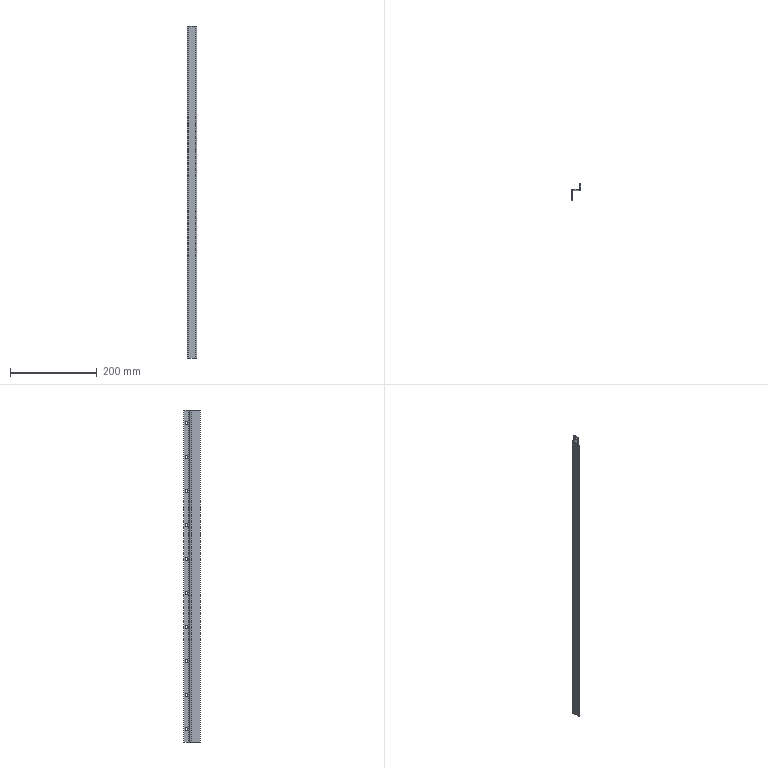Part | NX | features solid 2 | 1 solid | 34 faces | box 22 x 38 x 765 mm | volume 84234 mm3 | cylinder 24 | plane 10 | commonest cylinder face diameters 6 x20 4 x2 8 x2
STEP:
#1=CARTESIAN_POINT('',(2193.,-769.,290.));
#2=VERTEX_POINT('',#1);
#3=CARTESIAN_POINT('',(2191.,-769.,290.));
#4=VERTEX_POINT('',#3);
#5=CARTESIAN_POINT('',(2957.259,-769.,290.));
#6=DIRECTION('',(-1.,0.,0.));
#7=VECTOR('',#6,1000.);
#8=LINE('',#5,#7);
#9=EDGE_CURVE('',#2,#4,#8,.T.);
#10=ORIENTED_EDGE('',*,*,#9,.F.);
#11=CARTESIAN_POINT('',(2193.,-763.,290.));
#12=VERTEX_POINT('',#11);
#13=CARTESIAN_POINT('',(2193.,-766.,290.));
#14=DIRECTION('',(-1.,0.,0.));
#15=DIRECTION('',(0.,1.,0.));
#16=AXIS2_PLACEMENT_3D('',#13,#14,#15);
#17=CIRCLE('',#16,3.);
#18=EDGE_CURVE('',#12,#2,#17,.T.);
#19=ORIENTED_EDGE('',*,*,#18,.F.);
#20=CARTESIAN_POINT('',(2191.,-763.,290.));
#21=VERTEX_POINT('',#20);
#22=CARTESIAN_POINT('',(2957.259,-763.,290.));
#23=DIRECTION('',(-1.,0.,0.));
#24=VECTOR('',#23,1000.);
#25=LINE('',#22,#24);
#26=EDGE_CURVE('',#21,#12,#25,.F.);
#27=ORIENTED_EDGE('',*,*,#26,.F.);
#28=CARTESIAN_POINT('',(2191.,-766.,290.));
#29=DIRECTION('',(-1.,0.,0.));
#30=DIRECTION('',(0.,0.,1.));
#31=AXIS2_PLACEMENT_3D('',#28,#29,#30);
#32=CIRCLE('',#31,3.);
#33=EDGE_CURVE('',#21,#4,#32,.T.);
#34=ORIENTED_EDGE('',*,*,#33,.T.);
#35=EDGE_LOOP('',(#10,#19,#27,#34));
#36=FACE_BOUND('',#35,.T.);
#37=CARTESIAN_POINT('',(2957.259,-766.,290.));
#38=DIRECTION('',(-1.,0.,0.));
#39=DIRECTION('',(0.,1.,0.));
#40=AXIS2_PLACEMENT_3D('',#37,#38,#39);
#41=CYLINDRICAL_SURFACE('',#40,3.);
#42=ADVANCED_FACE('',(#36),#41,.F.);
#43=CARTESIAN_POINT('',(2173.,-777.,1025.));
#44=VERTEX_POINT('',#43);
#45=CARTESIAN_POINT('',(2173.,-798.,1025.));
#46=VERTEX_POINT('',#45);
#47=CARTESIAN_POINT('',(2173.,-775.,1025.));
#48=DIRECTION('',(0.,-1.,0.));
#49=VECTOR('',#48,1000.);
#50=LINE('',#47,#49);
#51=EDGE_CURVE('',#44,#46,#50,.T.);
#52=ORIENTED_EDGE('',*,*,#51,.T.);
#53=CARTESIAN_POINT('',(2173.,-798.,260.));
#54=VERTEX_POINT('',#53);
#55=CARTESIAN_POINT('',(2173.,-798.,260.));
#56=DIRECTION('',(0.,0.,1.));
#57=VECTOR('',#56,1000.);
#58=LINE('',#55,#57);
#59=EDGE_CURVE('',#54,#46,#58,.T.);
#60=ORIENTED_EDGE('',*,*,#59,.F.);
#61=CARTESIAN_POINT('',(2173.,-777.,260.));
#62=VERTEX_POINT('',#61);
#63=CARTESIAN_POINT('',(2173.,-775.,260.));
#64=DIRECTION('',(0.,-1.,0.));
#65=VECTOR('',#64,1000.);
#66=LINE('',#63,#65);
#67=EDGE_CURVE('',#62,#54,#66,.T.);
#68=ORIENTED_EDGE('',*,*,#67,.F.);
#69=CARTESIAN_POINT('',(2173.,-777.,260.));
#70=DIRECTION('',(0.,0.,1.));
#71=VECTOR('',#70,1000.);
#72=LINE('',#69,#71);
#73=EDGE_CURVE('',#62,#44,#72,.T.);
#74=ORIENTED_EDGE('',*,*,#73,.T.);
#75=EDGE_LOOP('',(#52,#60,#68,#74));
#76=FACE_BOUND('',#75,.T.);
#77=CARTESIAN_POINT('',(2173.,-775.,260.));
#78=DIRECTION('',(-1.,0.,0.));
#79=DIRECTION('',(0.,0.,1.));
#80=AXIS2_PLACEMENT_3D('',#77,#78,#79);
#81=PLANE('',#80);
#82=ADVANCED_FACE('',(#76),#81,.F.);
#83=CARTESIAN_POINT('',(2175.,-775.,1025.));
#84=VERTEX_POINT('',#83);
#85=CARTESIAN_POINT('',(2175.,-777.,1025.));
#86=DIRECTION('',(0.,0.,1.));
#87=DIRECTION('',(0.,1.,0.));
#88=AXIS2_PLACEMENT_3D('',#85,#86,#87);
#89=CIRCLE('',#88,2.);
#90=EDGE_CURVE('',#84,#44,#89,.T.);
#91=ORIENTED_EDGE('',*,*,#90,.T.);
#92=ORIENTED_EDGE('',*,*,#73,.F.);
#93=CARTESIAN_POINT('',(2175.,-775.,260.));
#94=VERTEX_POINT('',#93);
#95=CARTESIAN_POINT('',(2175.,-777.,260.));
#96=DIRECTION('',(0.,0.,1.));
#97=DIRECTION('',(0.,1.,0.));
#98=AXIS2_PLACEMENT_3D('',#95,#96,#97);
#99=CIRCLE('',#98,2.);
#100=EDGE_CURVE('',#94,#62,#99,.T.);
#101=ORIENTED_EDGE('',*,*,#100,.F.);
#102=CARTESIAN_POINT('',(2175.,-775.,260.));
#103=DIRECTION('',(0.,0.,1.));
#104=VECTOR('',#103,1000.);
#105=LINE('',#102,#104);
#106=EDGE_CURVE('',#94,#84,#105,.T.);
#107=ORIENTED_EDGE('',*,*,#106,.T.);
#108=EDGE_LOOP('',(#91,#92,#101,#107));
#109=FACE_BOUND('',#108,.T.);
#110=CARTESIAN_POINT('',(2175.,-777.,260.));
#111=DIRECTION('',(0.,0.,1.));
#112=DIRECTION('',(0.,-1.,0.));
#113=AXIS2_PLACEMENT_3D('',#110,#111,#112);
#114=CYLINDRICAL_SURFACE('',#113,2.);
#115=ADVANCED_FACE('',(#109),#114,.F.);
#116=CARTESIAN_POINT('',(2189.,-775.,1025.));
#117=VERTEX_POINT('',#116);
#118=CARTESIAN_POINT('',(2193.,-775.,1025.));
#119=DIRECTION('',(-1.,0.,0.));
#120=VECTOR('',#119,1000.);
#121=LINE('',#118,#120);
#122=EDGE_CURVE('',#117,#84,#121,.T.);
#123=ORIENTED_EDGE('',*,*,#122,.T.);
#124=ORIENTED_EDGE('',*,*,#106,.F.);
#125=CARTESIAN_POINT('',(2189.,-775.,260.));
#126=VERTEX_POINT('',#125);
#127=CARTESIAN_POINT('',(2193.,-775.,260.));
#128=DIRECTION('',(-1.,0.,0.));
#129=VECTOR('',#128,1000.);
#130=LINE('',#127,#129);
#131=EDGE_CURVE('',#126,#94,#130,.T.);
#132=ORIENTED_EDGE('',*,*,#131,.F.);
#133=CARTESIAN_POINT('',(2189.,-775.,260.));
#134=DIRECTION('',(0.,0.,1.));
#135=VECTOR('',#134,1000.);
#136=LINE('',#133,#135);
#137=EDGE_CURVE('',#126,#117,#136,.T.);
#138=ORIENTED_EDGE('',*,*,#137,.T.);
#139=EDGE_LOOP('',(#123,#124,#132,#138));
#140=FACE_BOUND('',#139,.T.);
#141=CARTESIAN_POINT('',(2193.,-775.,260.));
#142=DIRECTION('',(0.,1.,0.));
#143=DIRECTION('',(0.,0.,-1.));
#144=AXIS2_PLACEMENT_3D('',#141,#142,#143);
#145=PLANE('',#144);
#146=ADVANCED_FACE('',(#140),#145,.F.);
#147=CARTESIAN_POINT('',(2193.,-771.,1025.));
#148=VERTEX_POINT('',#147);
#149=CARTESIAN_POINT('',(2189.,-771.,1025.));
#150=DIRECTION('',(0.,0.,-1.));
#151=DIRECTION('',(0.,-1.,0.));
#152=AXIS2_PLACEMENT_3D('',#149,#150,#151);
#153=CIRCLE('',#152,4.);
#154=EDGE_CURVE('',#148,#117,#153,.T.);
#155=ORIENTED_EDGE('',*,*,#154,.T.);
#156=ORIENTED_EDGE('',*,*,#137,.F.);
#157=CARTESIAN_POINT('',(2193.,-771.,260.));
#158=VERTEX_POINT('',#157);
#159=CARTESIAN_POINT('',(2189.,-771.,260.));
#160=DIRECTION('',(0.,0.,-1.));
#161=DIRECTION('',(0.,-1.,0.));
#162=AXIS2_PLACEMENT_3D('',#159,#160,#161);
#163=CIRCLE('',#162,4.);
#164=EDGE_CURVE('',#158,#126,#163,.T.);
#165=ORIENTED_EDGE('',*,*,#164,.F.);
#166=CARTESIAN_POINT('',(2193.,-771.,260.));
#167=DIRECTION('',(0.,0.,1.));
#168=VECTOR('',#167,1000.);
#169=LINE('',#166,#168);
#170=EDGE_CURVE('',#158,#148,#169,.T.);
#171=ORIENTED_EDGE('',*,*,#170,.T.);
#172=EDGE_LOOP('',(#155,#156,#165,#171));
#173=FACE_BOUND('',#172,.T.);
#174=CARTESIAN_POINT('',(2189.,-771.,260.));
#175=DIRECTION('',(0.,0.,1.));
#176=DIRECTION('',(0.,-1.,0.));
#177=AXIS2_PLACEMENT_3D('',#174,#175,#176);
#178=CYLINDRICAL_SURFACE('',#177,4.);
#179=ADVANCED_FACE('',(#173),#178,.T.);
#180=ORIENTED_EDGE('',*,*,#18,.T.);
#181=CARTESIAN_POINT('',(2193.,-766.,290.));
#182=DIRECTION('',(-1.,0.,0.));
#183=DIRECTION('',(0.,1.,0.));
#184=AXIS2_PLACEMENT_3D('',#181,#182,#183);
#185=CIRCLE('',#184,3.);
#186=EDGE_CURVE('',#2,#12,#185,.T.);
#187=ORIENTED_EDGE('',*,*,#186,.T.);
#188=EDGE_LOOP('',(#180,#187));
#189=FACE_BOUND('',#188,.T.);
#190=CARTESIAN_POINT('',(2193.,-763.,368.333));
#191=VERTEX_POINT('',#190);
#192=CARTESIAN_POINT('',(2193.,-769.,368.333));
#193=VERTEX_POINT('',#192);
#194=CARTESIAN_POINT('',(2193.,-766.,368.333));
#195=DIRECTION('',(-1.,0.,0.));
#196=DIRECTION('',(0.,1.,0.));
#197=AXIS2_PLACEMENT_3D('',#194,#195,#196);
#198=CIRCLE('',#197,3.);
#199=EDGE_CURVE('',#191,#193,#198,.T.);
#200=ORIENTED_EDGE('',*,*,#199,.T.);
#201=CARTESIAN_POINT('',(2193.,-766.,368.333));
#202=DIRECTION('',(-1.,0.,0.));
#203=DIRECTION('',(0.,1.,0.));
#204=AXIS2_PLACEMENT_3D('',#201,#202,#203);
#205=CIRCLE('',#204,3.);
#206=EDGE_CURVE('',#193,#191,#205,.T.);
#207=ORIENTED_EDGE('',*,*,#206,.T.);
#208=EDGE_LOOP('',(#200,#207));
#209=FACE_BOUND('',#208,.T.);
#210=CARTESIAN_POINT('',(2193.,-763.,446.667));
#211=VERTEX_POINT('',#210);
#212=CARTESIAN_POINT('',(2193.,-769.,446.667));
#213=VERTEX_POINT('',#212);
#214=CARTESIAN_POINT('',(2193.,-766.,446.667));
#215=DIRECTION('',(-1.,0.,0.));
#216=DIRECTION('',(0.,1.,0.));
#217=AXIS2_PLACEMENT_3D('',#214,#215,#216);
#218=CIRCLE('',#217,3.);
#219=EDGE_CURVE('',#211,#213,#218,.T.);
#220=ORIENTED_EDGE('',*,*,#219,.T.);
#221=CARTESIAN_POINT('',(2193.,-766.,446.667));
#222=DIRECTION('',(-1.,0.,0.));
#223=DIRECTION('',(0.,1.,0.));
#224=AXIS2_PLACEMENT_3D('',#221,#222,#223);
#225=CIRCLE('',#224,3.);
#226=EDGE_CURVE('',#213,#211,#225,.T.);
#227=ORIENTED_EDGE('',*,*,#226,.T.);
#228=EDGE_LOOP('',(#220,#227));
#229=FACE_BOUND('',#228,.T.);
#230=CARTESIAN_POINT('',(2193.,-763.,525.));
#231=VERTEX_POINT('',#230);
#232=CARTESIAN_POINT('',(2193.,-769.,525.));
#233=VERTEX_POINT('',#232);
#234=CARTESIAN_POINT('',(2193.,-766.,525.));
#235=DIRECTION('',(-1.,0.,0.));
#236=DIRECTION('',(0.,1.,0.));
#237=AXIS2_PLACEMENT_3D('',#234,#235,#236);
#238=CIRCLE('',#237,3.);
#239=EDGE_CURVE('',#231,#233,#238,.T.);
#240=ORIENTED_EDGE('',*,*,#239,.T.);
#241=CARTESIAN_POINT('',(2193.,-766.,525.));
#242=DIRECTION('',(-1.,0.,0.));
#243=DIRECTION('',(0.,1.,0.));
#244=AXIS2_PLACEMENT_3D('',#241,#242,#243);
#245=CIRCLE('',#244,3.);
#246=EDGE_CURVE('',#233,#231,#245,.T.);
#247=ORIENTED_EDGE('',*,*,#246,.T.);
#248=EDGE_LOOP('',(#240,#247));
#249=FACE_BOUND('',#248,.T.);
#250=CARTESIAN_POINT('',(2193.,-763.,603.333));
#251=VERTEX_POINT('',#250);
#252=CARTESIAN_POINT('',(2193.,-769.,603.333));
#253=VERTEX_POINT('',#252);
#254=CARTESIAN_POINT('',(2193.,-766.,603.333));
#255=DIRECTION('',(-1.,0.,0.));
#256=DIRECTION('',(0.,1.,0.));
#257=AXIS2_PLACEMENT_3D('',#254,#255,#256);
#258=CIRCLE('',#257,3.);
#259=EDGE_CURVE('',#251,#253,#258,.T.);
#260=ORIENTED_EDGE('',*,*,#259,.T.);
#261=CARTESIAN_POINT('',(2193.,-766.,603.333));
#262=DIRECTION('',(-1.,0.,0.));
#263=DIRECTION('',(0.,1.,0.));
#264=AXIS2_PLACEMENT_3D('',#261,#262,#263);
#265=CIRCLE('',#264,3.);
#266=EDGE_CURVE('',#253,#251,#265,.T.);
#267=ORIENTED_EDGE('',*,*,#266,.T.);
#268=EDGE_LOOP('',(#260,#267));
#269=FACE_BOUND('',#268,.T.);
#270=CARTESIAN_POINT('',(2193.,-763.,681.667));
#271=VERTEX_POINT('',#270);
#272=CARTESIAN_POINT('',(2193.,-769.,681.667));
#273=VERTEX_POINT('',#272);
#274=CARTESIAN_POINT('',(2193.,-766.,681.667));
#275=DIRECTION('',(-1.,0.,0.));
#276=DIRECTION('',(0.,1.,0.));
#277=AXIS2_PLACEMENT_3D('',#274,#275,#276);
#278=CIRCLE('',#277,3.);
#279=EDGE_CURVE('',#271,#273,#278,.T.);
#280=ORIENTED_EDGE('',*,*,#279,.T.);
#281=CARTESIAN_POINT('',(2193.,-766.,681.667));
#282=DIRECTION('',(-1.,0.,0.));
#283=DIRECTION('',(0.,1.,0.));
#284=AXIS2_PLACEMENT_3D('',#281,#282,#283);
#285=CIRCLE('',#284,3.);
#286=EDGE_CURVE('',#273,#271,#285,.T.);
#287=ORIENTED_EDGE('',*,*,#286,.T.);
#288=EDGE_LOOP('',(#280,#287));
#289=FACE_BOUND('',#288,.T.);
#290=CARTESIAN_POINT('',(2193.,-763.,760.));
#291=VERTEX_POINT('',#290);
#292=CARTESIAN_POINT('',(2193.,-769.,760.));
#293=VERTEX_POINT('',#292);
#294=CARTESIAN_POINT('',(2193.,-766.,760.));
#295=DIRECTION('',(-1.,0.,0.));
#296=DIRECTION('',(0.,1.,0.));
#297=AXIS2_PLACEMENT_3D('',#294,#295,#296);
#298=CIRCLE('',#297,3.);
#299=EDGE_CURVE('',#291,#293,#298,.T.);
#300=ORIENTED_EDGE('',*,*,#299,.T.);
#301=CARTESIAN_POINT('',(2193.,-766.,760.));
#302=DIRECTION('',(-1.,0.,0.));
#303=DIRECTION('',(0.,1.,0.));
#304=AXIS2_PLACEMENT_3D('',#301,#302,#303);
#305=CIRCLE('',#304,3.);
#306=EDGE_CURVE('',#293,#291,#305,.T.);
#307=ORIENTED_EDGE('',*,*,#306,.T.);
#308=EDGE_LOOP('',(#300,#307));
#309=FACE_BOUND('',#308,.T.);
#310=CARTESIAN_POINT('',(2193.,-763.,838.333));
#311=VERTEX_POINT('',#310);
#312=CARTESIAN_POINT('',(2193.,-769.,838.333));
#313=VERTEX_POINT('',#312);
#314=CARTESIAN_POINT('',(2193.,-766.,838.333));
#315=DIRECTION('',(-1.,0.,0.));
#316=DIRECTION('',(0.,1.,0.));
#317=AXIS2_PLACEMENT_3D('',#314,#315,#316);
#318=CIRCLE('',#317,3.);
#319=EDGE_CURVE('',#311,#313,#318,.T.);
#320=ORIENTED_EDGE('',*,*,#319,.T.);
#321=CARTESIAN_POINT('',(2193.,-766.,838.333));
#322=DIRECTION('',(-1.,0.,0.));
#323=DIRECTION('',(0.,1.,0.));
#324=AXIS2_PLACEMENT_3D('',#321,#322,#323);
#325=CIRCLE('',#324,3.);
#326=EDGE_CURVE('',#313,#311,#325,.T.);
#327=ORIENTED_EDGE('',*,*,#326,.T.);
#328=EDGE_LOOP('',(#320,#327));
#329=FACE_BOUND('',#328,.T.);
#330=CARTESIAN_POINT('',(2193.,-763.,916.667));
#331=VERTEX_POINT('',#330);
#332=CARTESIAN_POINT('',(2193.,-769.,916.667));
#333=VERTEX_POINT('',#332);
#334=CARTESIAN_POINT('',(2193.,-766.,916.667));
#335=DIRECTION('',(-1.,0.,0.));
#336=DIRECTION('',(0.,1.,0.));
#337=AXIS2_PLACEMENT_3D('',#334,#335,#336);
#338=CIRCLE('',#337,3.);
#339=EDGE_CURVE('',#331,#333,#338,.T.);
#340=ORIENTED_EDGE('',*,*,#339,.T.);
#341=CARTESIAN_POINT('',(2193.,-766.,916.667));
#342=DIRECTION('',(-1.,0.,0.));
#343=DIRECTION('',(0.,1.,0.));
#344=AXIS2_PLACEMENT_3D('',#341,#342,#343);
#345=CIRCLE('',#344,3.);
#346=EDGE_CURVE('',#333,#331,#345,.T.);
#347=ORIENTED_EDGE('',*,*,#346,.T.);
#348=EDGE_LOOP('',(#340,#347));
#349=FACE_BOUND('',#348,.T.);
#350=CARTESIAN_POINT('',(2193.,-763.,995.));
#351=VERTEX_POINT('',#350);
#352=CARTESIAN_POINT('',(2193.,-769.,995.));
#353=VERTEX_POINT('',#352);
#354=CARTESIAN_POINT('',(2193.,-766.,995.));
#355=DIRECTION('',(-1.,0.,0.));
#356=DIRECTION('',(0.,1.,0.));
#357=AXIS2_PLACEMENT_3D('',#354,#355,#356);
#358=CIRCLE('',#357,3.);
#359=EDGE_CURVE('',#351,#353,#358,.T.);
#360=ORIENTED_EDGE('',*,*,#359,.T.);
#361=CARTESIAN_POINT('',(2193.,-766.,995.));
#362=DIRECTION('',(-1.,0.,0.));
#363=DIRECTION('',(0.,1.,0.));
#364=AXIS2_PLACEMENT_3D('',#361,#362,#363);
#365=CIRCLE('',#364,3.);
#366=EDGE_CURVE('',#353,#351,#365,.T.);
#367=ORIENTED_EDGE('',*,*,#366,.T.);
#368=EDGE_LOOP('',(#360,#367));
#369=FACE_BOUND('',#368,.T.);
#370=CARTESIAN_POINT('',(2193.,-760.,1025.));
#371=VERTEX_POINT('',#370);
#372=CARTESIAN_POINT('',(2193.,-760.,1025.));
#373=DIRECTION('',(0.,-1.,0.));
#374=VECTOR('',#373,1000.);
#375=LINE('',#372,#374);
#376=EDGE_CURVE('',#371,#148,#375,.T.);
#377=ORIENTED_EDGE('',*,*,#376,.T.);
#378=ORIENTED_EDGE('',*,*,#170,.F.);
#379=CARTESIAN_POINT('',(2193.,-760.,260.));
#380=VERTEX_POINT('',#379);
#381=CARTESIAN_POINT('',(2193.,-760.,260.));
#382=DIRECTION('',(0.,-1.,0.));
#383=VECTOR('',#382,1000.);
#384=LINE('',#381,#383);
#385=EDGE_CURVE('',#380,#158,#384,.T.);
#386=ORIENTED_EDGE('',*,*,#385,.F.);
#387=CARTESIAN_POINT('',(2193.,-760.,260.));
#388=DIRECTION('',(0.,0.,1.));
#389=VECTOR('',#388,1000.);
#390=LINE('',#387,#389);
#391=EDGE_CURVE('',#380,#371,#390,.T.);
#392=ORIENTED_EDGE('',*,*,#391,.T.);
#393=EDGE_LOOP('',(#377,#378,#386,#392));
#394=FACE_BOUND('',#393,.T.);
#395=CARTESIAN_POINT('',(2193.,-760.,260.));
#396=DIRECTION('',(-1.,0.,0.));
#397=DIRECTION('',(0.,0.,1.));
#398=AXIS2_PLACEMENT_3D('',#395,#396,#397);
#399=PLANE('',#398);
#400=ADVANCED_FACE('',(#189,#209,#229,#249,#269,#289,#309,#329,#349,#369,#394),#399,.F.);
#401=CARTESIAN_POINT('',(2171.,-777.,1025.));
#402=VERTEX_POINT('',#401);
#403=CARTESIAN_POINT('',(2171.,-798.,1025.));
#404=VERTEX_POINT('',#403);
#405=CARTESIAN_POINT('',(2171.,-775.,1025.));
#406=DIRECTION('',(0.,-1.,0.));
#407=VECTOR('',#406,1000.);
#408=LINE('',#405,#407);
#409=EDGE_CURVE('',#402,#404,#408,.T.);
#410=ORIENTED_EDGE('',*,*,#409,.F.);
#411=CARTESIAN_POINT('',(2171.,-777.,260.));
#412=VERTEX_POINT('',#411);
#413=CARTESIAN_POINT('',(2171.,-777.,260.));
#414=DIRECTION('',(0.,0.,1.));
#415=VECTOR('',#414,1000.);
#416=LINE('',#413,#415);
#417=EDGE_CURVE('',#412,#402,#416,.T.);
#418=ORIENTED_EDGE('',*,*,#417,.F.);
#419=CARTESIAN_POINT('',(2171.,-798.,260.));
#420=VERTEX_POINT('',#419);
#421=CARTESIAN_POINT('',(2171.,-775.,260.));
#422=DIRECTION('',(0.,-1.,0.));
#423=VECTOR('',#422,1000.);
#424=LINE('',#421,#423);
#425=EDGE_CURVE('',#412,#420,#424,.T.);
#426=ORIENTED_EDGE('',*,*,#425,.T.);
#427=CARTESIAN_POINT('',(2171.,-798.,260.));
#428=DIRECTION('',(0.,0.,1.));
#429=VECTOR('',#428,1000.);
#430=LINE('',#427,#429);
#431=EDGE_CURVE('',#420,#404,#430,.T.);
#432=ORIENTED_EDGE('',*,*,#431,.T.);
#433=EDGE_LOOP('',(#410,#418,#426,#432));
#434=FACE_BOUND('',#433,.T.);
#435=CARTESIAN_POINT('',(2171.,-775.,260.));
#436=DIRECTION('',(-1.,0.,0.));
#437=DIRECTION('',(0.,0.,1.));
#438=AXIS2_PLACEMENT_3D('',#435,#436,#437);
#439=PLANE('',#438);
#440=ADVANCED_FACE('',(#434),#439,.T.);
#441=CARTESIAN_POINT('',(2175.,-773.,1025.));
#442=VERTEX_POINT('',#441);
#443=CARTESIAN_POINT('',(2175.,-777.,1025.));
#444=DIRECTION('',(0.,0.,1.));
#445=DIRECTION('',(0.,-1.,0.));
#446=AXIS2_PLACEMENT_3D('',#443,#444,#445);
#447=CIRCLE('',#446,4.);
#448=EDGE_CURVE('',#442,#402,#447,.T.);
#449=ORIENTED_EDGE('',*,*,#448,.F.);
#450=CARTESIAN_POINT('',(2175.,-773.,260.));
#451=VERTEX_POINT('',#450);
#452=CARTESIAN_POINT('',(2175.,-773.,260.));
#453=DIRECTION('',(0.,0.,1.));
#454=VECTOR('',#453,1000.);
#455=LINE('',#452,#454);
#456=EDGE_CURVE('',#451,#442,#455,.T.);
#457=ORIENTED_EDGE('',*,*,#456,.F.);
#458=CARTESIAN_POINT('',(2175.,-777.,260.));
#459=DIRECTION('',(0.,0.,1.));
#460=DIRECTION('',(0.,-1.,0.));
#461=AXIS2_PLACEMENT_3D('',#458,#459,#460);
#462=CIRCLE('',#461,4.);
#463=EDGE_CURVE('',#451,#412,#462,.T.);
#464=ORIENTED_EDGE('',*,*,#463,.T.);
#465=ORIENTED_EDGE('',*,*,#417,.T.);
#466=EDGE_LOOP('',(#449,#457,#464,#465));
#467=FACE_BOUND('',#466,.T.);
#468=CARTESIAN_POINT('',(2175.,-777.,260.));
#469=DIRECTION('',(0.,0.,1.));
#470=DIRECTION('',(0.,-1.,0.));
#471=AXIS2_PLACEMENT_3D('',#468,#469,#470);
#472=CYLINDRICAL_SURFACE('',#471,4.);
#473=ADVANCED_FACE('',(#467),#472,.T.);
#474=CARTESIAN_POINT('',(2189.,-773.,1025.));
#475=VERTEX_POINT('',#474);
#476=CARTESIAN_POINT('',(2193.,-773.,1025.));
#477=DIRECTION('',(-1.,0.,0.));
#478=VECTOR('',#477,1000.);
#479=LINE('',#476,#478);
#480=EDGE_CURVE('',#475,#442,#479,.T.);
#481=ORIENTED_EDGE('',*,*,#480,.F.);
#482=CARTESIAN_POINT('',(2189.,-773.,260.));
#483=VERTEX_POINT('',#482);
#484=CARTESIAN_POINT('',(2189.,-773.,260.));
#485=DIRECTION('',(0.,0.,1.));
#486=VECTOR('',#485,1000.);
#487=LINE('',#484,#486);
#488=EDGE_CURVE('',#483,#475,#487,.T.);
#489=ORIENTED_EDGE('',*,*,#488,.F.);
#490=CARTESIAN_POINT('',(2193.,-773.,260.));
#491=DIRECTION('',(-1.,0.,0.));
#492=VECTOR('',#491,1000.);
#493=LINE('',#490,#492);
#494=EDGE_CURVE('',#483,#451,#493,.T.);
#495=ORIENTED_EDGE('',*,*,#494,.T.);
#496=ORIENTED_EDGE('',*,*,#456,.T.);
#497=EDGE_LOOP('',(#481,#489,#495,#496));
#498=FACE_BOUND('',#497,.T.);
#499=CARTESIAN_POINT('',(2193.,-773.,260.));
#500=DIRECTION('',(0.,1.,0.));
#501=DIRECTION('',(0.,0.,-1.));
#502=AXIS2_PLACEMENT_3D('',#499,#500,#501);
#503=PLANE('',#502);
#504=ADVANCED_FACE('',(#498),#503,.T.);
#505=CARTESIAN_POINT('',(2191.,-771.,1025.));
#506=VERTEX_POINT('',#505);
#507=CARTESIAN_POINT('',(2189.,-771.,1025.));
#508=DIRECTION('',(0.,0.,-1.));
#509=DIRECTION('',(0.,-1.,0.));
#510=AXIS2_PLACEMENT_3D('',#507,#508,#509);
#511=CIRCLE('',#510,2.);
#512=EDGE_CURVE('',#506,#475,#511,.T.);
#513=ORIENTED_EDGE('',*,*,#512,.F.);
#514=CARTESIAN_POINT('',(2191.,-771.,260.));
#515=VERTEX_POINT('',#514);
#516=CARTESIAN_POINT('',(2191.,-771.,260.));
#517=DIRECTION('',(0.,0.,1.));
#518=VECTOR('',#517,1000.);
#519=LINE('',#516,#518);
#520=EDGE_CURVE('',#515,#506,#519,.T.);
#521=ORIENTED_EDGE('',*,*,#520,.F.);
#522=CARTESIAN_POINT('',(2189.,-771.,260.));
#523=DIRECTION('',(0.,0.,-1.));
#524=DIRECTION('',(0.,-1.,0.));
#525=AXIS2_PLACEMENT_3D('',#522,#523,#524);
#526=CIRCLE('',#525,2.);
#527=EDGE_CURVE('',#515,#483,#526,.T.);
#528=ORIENTED_EDGE('',*,*,#527,.T.);
#529=ORIENTED_EDGE('',*,*,#488,.T.);
#530=EDGE_LOOP('',(#513,#521,#528,#529));
#531=FACE_BOUND('',#530,.T.);
#532=CARTESIAN_POINT('',(2189.,-771.,260.));
#533=DIRECTION('',(0.,0.,1.));
#534=DIRECTION('',(0.,-1.,0.));
#535=AXIS2_PLACEMENT_3D('',#532,#533,#534);
#536=CYLINDRICAL_SURFACE('',#535,2.);
#537=ADVANCED_FACE('',(#531),#536,.F.);
#538=ORIENTED_EDGE('',*,*,#33,.F.);
#539=CARTESIAN_POINT('',(2191.,-766.,290.));
#540=DIRECTION('',(-1.,0.,0.));
#541=DIRECTION('',(0.,0.,1.));
#542=AXIS2_PLACEMENT_3D('',#539,#540,#541);
#543=CIRCLE('',#542,3.);
#544=EDGE_CURVE('',#4,#21,#543,.T.);
#545=ORIENTED_EDGE('',*,*,#544,.F.);
#546=EDGE_LOOP('',(#538,#545));
#547=FACE_BOUND('',#546,.T.);
#548=CARTESIAN_POINT('',(2191.,-763.,368.333));
#549=VERTEX_POINT('',#548);
#550=CARTESIAN_POINT('',(2191.,-769.,368.333));
#551=VERTEX_POINT('',#550);
#552=CARTESIAN_POINT('',(2191.,-766.,368.333));
#553=DIRECTION('',(-1.,0.,0.));
#554=DIRECTION('',(0.,0.,1.));
#555=AXIS2_PLACEMENT_3D('',#552,#553,#554);
#556=CIRCLE('',#555,3.);
#557=EDGE_CURVE('',#549,#551,#556,.T.);
#558=ORIENTED_EDGE('',*,*,#557,.F.);
#559=CARTESIAN_POINT('',(2191.,-766.,368.333));
#560=DIRECTION('',(-1.,0.,0.));
#561=DIRECTION('',(0.,0.,1.));
#562=AXIS2_PLACEMENT_3D('',#559,#560,#561);
#563=CIRCLE('',#562,3.);
#564=EDGE_CURVE('',#551,#549,#563,.T.);
#565=ORIENTED_EDGE('',*,*,#564,.F.);
#566=EDGE_LOOP('',(#558,#565));
#567=FACE_BOUND('',#566,.T.);
#568=CARTESIAN_POINT('',(2191.,-763.,446.667));
#569=VERTEX_POINT('',#568);
#570=CARTESIAN_POINT('',(2191.,-769.,446.667));
#571=VERTEX_POINT('',#570);
#572=CARTESIAN_POINT('',(2191.,-766.,446.667));
#573=DIRECTION('',(-1.,0.,0.));
#574=DIRECTION('',(0.,0.,1.));
#575=AXIS2_PLACEMENT_3D('',#572,#573,#574);
#576=CIRCLE('',#575,3.);
#577=EDGE_CURVE('',#569,#571,#576,.T.);
#578=ORIENTED_EDGE('',*,*,#577,.F.);
#579=CARTESIAN_POINT('',(2191.,-766.,446.667));
#580=DIRECTION('',(-1.,0.,0.));
#581=DIRECTION('',(0.,0.,1.));
#582=AXIS2_PLACEMENT_3D('',#579,#580,#581);
#583=CIRCLE('',#582,3.);
#584=EDGE_CURVE('',#571,#569,#583,.T.);
#585=ORIENTED_EDGE('',*,*,#584,.F.);
#586=EDGE_LOOP('',(#578,#585));
#587=FACE_BOUND('',#586,.T.);
#588=CARTESIAN_POINT('',(2191.,-763.,525.));
#589=VERTEX_POINT('',#588);
#590=CARTESIAN_POINT('',(2191.,-769.,525.));
#591=VERTEX_POINT('',#590);
#592=CARTESIAN_POINT('',(2191.,-766.,525.));
#593=DIRECTION('',(-1.,0.,0.));
#594=DIRECTION('',(0.,0.,1.));
#595=AXIS2_PLACEMENT_3D('',#592,#593,#594);
#596=CIRCLE('',#595,3.);
#597=EDGE_CURVE('',#589,#591,#596,.T.);
#598=ORIENTED_EDGE('',*,*,#597,.F.);
#599=CARTESIAN_POINT('',(2191.,-766.,525.));
#600=DIRECTION('',(-1.,0.,0.));
#601=DIRECTION('',(0.,0.,1.));
#602=AXIS2_PLACEMENT_3D('',#599,#600,#601);
#603=CIRCLE('',#602,3.);
#604=EDGE_CURVE('',#591,#589,#603,.T.);
#605=ORIENTED_EDGE('',*,*,#604,.F.);
#606=EDGE_LOOP('',(#598,#605));
#607=FACE_BOUND('',#606,.T.);
#608=CARTESIAN_POINT('',(2191.,-763.,603.333));
#609=VERTEX_POINT('',#608);
#610=CARTESIAN_POINT('',(2191.,-769.,603.333));
#611=VERTEX_POINT('',#610);
#612=CARTESIAN_POINT('',(2191.,-766.,603.333));
#613=DIRECTION('',(-1.,0.,0.));
#614=DIRECTION('',(0.,0.,1.));
#615=AXIS2_PLACEMENT_3D('',#612,#613,#614);
#616=CIRCLE('',#615,3.);
#617=EDGE_CURVE('',#609,#611,#616,.T.);
#618=ORIENTED_EDGE('',*,*,#617,.F.);
#619=CARTESIAN_POINT('',(2191.,-766.,603.333));
#620=DIRECTION('',(-1.,0.,0.));
#621=DIRECTION('',(0.,0.,1.));
#622=AXIS2_PLACEMENT_3D('',#619,#620,#621);
#623=CIRCLE('',#622,3.);
#624=EDGE_CURVE('',#611,#609,#623,.T.);
#625=ORIENTED_EDGE('',*,*,#624,.F.);
#626=EDGE_LOOP('',(#618,#625));
#627=FACE_BOUND('',#626,.T.);
#628=CARTESIAN_POINT('',(2191.,-763.,681.667));
#629=VERTEX_POINT('',#628);
#630=CARTESIAN_POINT('',(2191.,-769.,681.667));
#631=VERTEX_POINT('',#630);
#632=CARTESIAN_POINT('',(2191.,-766.,681.667));
#633=DIRECTION('',(-1.,0.,0.));
#634=DIRECTION('',(0.,0.,1.));
#635=AXIS2_PLACEMENT_3D('',#632,#633,#634);
#636=CIRCLE('',#635,3.);
#637=EDGE_CURVE('',#629,#631,#636,.T.);
#638=ORIENTED_EDGE('',*,*,#637,.F.);
#639=CARTESIAN_POINT('',(2191.,-766.,681.667));
#640=DIRECTION('',(-1.,0.,0.));
#641=DIRECTION('',(0.,0.,1.));
#642=AXIS2_PLACEMENT_3D('',#639,#640,#641);
#643=CIRCLE('',#642,3.);
#644=EDGE_CURVE('',#631,#629,#643,.T.);
#645=ORIENTED_EDGE('',*,*,#644,.F.);
#646=EDGE_LOOP('',(#638,#645));
#647=FACE_BOUND('',#646,.T.);
#648=CARTESIAN_POINT('',(2191.,-763.,760.));
#649=VERTEX_POINT('',#648);
#650=CARTESIAN_POINT('',(2191.,-769.,760.));
#651=VERTEX_POINT('',#650);
#652=CARTESIAN_POINT('',(2191.,-766.,760.));
#653=DIRECTION('',(-1.,0.,0.));
#654=DIRECTION('',(0.,0.,1.));
#655=AXIS2_PLACEMENT_3D('',#652,#653,#654);
#656=CIRCLE('',#655,3.);
#657=EDGE_CURVE('',#649,#651,#656,.T.);
#658=ORIENTED_EDGE('',*,*,#657,.F.);
#659=CARTESIAN_POINT('',(2191.,-766.,760.));
#660=DIRECTION('',(-1.,0.,0.));
#661=DIRECTION('',(0.,0.,1.));
#662=AXIS2_PLACEMENT_3D('',#659,#660,#661);
#663=CIRCLE('',#662,3.);
#664=EDGE_CURVE('',#651,#649,#663,.T.);
#665=ORIENTED_EDGE('',*,*,#664,.F.);
#666=EDGE_LOOP('',(#658,#665));
#667=FACE_BOUND('',#666,.T.);
#668=CARTESIAN_POINT('',(2191.,-763.,838.333));
#669=VERTEX_POINT('',#668);
#670=CARTESIAN_POINT('',(2191.,-769.,838.333));
#671=VERTEX_POINT('',#670);
#672=CARTESIAN_POINT('',(2191.,-766.,838.333));
#673=DIRECTION('',(-1.,0.,0.));
#674=DIRECTION('',(0.,0.,1.));
#675=AXIS2_PLACEMENT_3D('',#672,#673,#674);
#676=CIRCLE('',#675,3.);
#677=EDGE_CURVE('',#669,#671,#676,.T.);
#678=ORIENTED_EDGE('',*,*,#677,.F.);
#679=CARTESIAN_POINT('',(2191.,-766.,838.333));
#680=DIRECTION('',(-1.,0.,0.));
#681=DIRECTION('',(0.,0.,1.));
#682=AXIS2_PLACEMENT_3D('',#679,#680,#681);
#683=CIRCLE('',#682,3.);
#684=EDGE_CURVE('',#671,#669,#683,.T.);
#685=ORIENTED_EDGE('',*,*,#684,.F.);
#686=EDGE_LOOP('',(#678,#685));
#687=FACE_BOUND('',#686,.T.);
#688=CARTESIAN_POINT('',(2191.,-763.,916.667));
#689=VERTEX_POINT('',#688);
#690=CARTESIAN_POINT('',(2191.,-769.,916.667));
#691=VERTEX_POINT('',#690);
#692=CARTESIAN_POINT('',(2191.,-766.,916.667));
#693=DIRECTION('',(-1.,0.,0.));
#694=DIRECTION('',(0.,0.,1.));
#695=AXIS2_PLACEMENT_3D('',#692,#693,#694);
#696=CIRCLE('',#695,3.);
#697=EDGE_CURVE('',#689,#691,#696,.T.);
#698=ORIENTED_EDGE('',*,*,#697,.F.);
#699=CARTESIAN_POINT('',(2191.,-766.,916.667));
#700=DIRECTION('',(-1.,0.,0.));
#701=DIRECTION('',(0.,0.,1.));
#702=AXIS2_PLACEMENT_3D('',#699,#700,#701);
#703=CIRCLE('',#702,3.);
#704=EDGE_CURVE('',#691,#689,#703,.T.);
#705=ORIENTED_EDGE('',*,*,#704,.F.);
#706=EDGE_LOOP('',(#698,#705));
#707=FACE_BOUND('',#706,.T.);
#708=CARTESIAN_POINT('',(2191.,-763.,995.));
#709=VERTEX_POINT('',#708);
#710=CARTESIAN_POINT('',(2191.,-769.,995.));
#711=VERTEX_POINT('',#710);
#712=CARTESIAN_POINT('',(2191.,-766.,995.));
#713=DIRECTION('',(-1.,0.,0.));
#714=DIRECTION('',(0.,0.,1.));
#715=AXIS2_PLACEMENT_3D('',#712,#713,#714);
#716=CIRCLE('',#715,3.);
#717=EDGE_CURVE('',#709,#711,#716,.T.);
#718=ORIENTED_EDGE('',*,*,#717,.F.);
#719=CARTESIAN_POINT('',(2191.,-766.,995.));
#720=DIRECTION('',(-1.,0.,0.));
#721=DIRECTION('',(0.,0.,1.));
#722=AXIS2_PLACEMENT_3D('',#719,#720,#721);
#723=CIRCLE('',#722,3.);
#724=EDGE_CURVE('',#711,#709,#723,.T.);
#725=ORIENTED_EDGE('',*,*,#724,.F.);
#726=EDGE_LOOP('',(#718,#725));
#727=FACE_BOUND('',#726,.T.);
#728=CARTESIAN_POINT('',(2191.,-760.,1025.));
#729=VERTEX_POINT('',#728);
#730=CARTESIAN_POINT('',(2191.,-760.,1025.));
#731=DIRECTION('',(0.,-1.,0.));
#732=VECTOR('',#731,1000.);
#733=LINE('',#730,#732);
#734=EDGE_CURVE('',#729,#506,#733,.T.);
#735=ORIENTED_EDGE('',*,*,#734,.F.);
#736=CARTESIAN_POINT('',(2191.,-760.,260.));
#737=VERTEX_POINT('',#736);
#738=CARTESIAN_POINT('',(2191.,-760.,260.));
#739=DIRECTION('',(0.,0.,1.));
#740=VECTOR('',#739,1000.);
#741=LINE('',#738,#740);
#742=EDGE_CURVE('',#737,#729,#741,.T.);
#743=ORIENTED_EDGE('',*,*,#742,.F.);
#744=CARTESIAN_POINT('',(2191.,-760.,260.));
#745=DIRECTION('',(0.,-1.,0.));
#746=VECTOR('',#745,1000.);
#747=LINE('',#744,#746);
#748=EDGE_CURVE('',#737,#515,#747,.T.);
#749=ORIENTED_EDGE('',*,*,#748,.T.);
#750=ORIENTED_EDGE('',*,*,#520,.T.);
#751=EDGE_LOOP('',(#735,#743,#749,#750));
#752=FACE_BOUND('',#751,.T.);
#753=CARTESIAN_POINT('',(2191.,-760.,260.));
#754=DIRECTION('',(-1.,0.,0.));
#755=DIRECTION('',(0.,0.,1.));
#756=AXIS2_PLACEMENT_3D('',#753,#754,#755);
#757=PLANE('',#756);
#758=ADVANCED_FACE('',(#547,#567,#587,#607,#627,#647,#667,#687,#707,#727,#752),#757,.T.);
#759=ORIENTED_EDGE('',*,*,#391,.F.);
#760=CARTESIAN_POINT('',(2193.,-760.,260.));
#761=DIRECTION('',(-1.,0.,0.));
#762=VECTOR('',#761,1000.);
#763=LINE('',#760,#762);
#764=EDGE_CURVE('',#380,#737,#763,.T.);
#765=ORIENTED_EDGE('',*,*,#764,.T.);
#766=ORIENTED_EDGE('',*,*,#742,.T.);
#767=CARTESIAN_POINT('',(2193.,-760.,1025.));
#768=DIRECTION('',(-1.,0.,0.));
#769=VECTOR('',#768,1000.);
#770=LINE('',#767,#769);
#771=EDGE_CURVE('',#371,#729,#770,.T.);
#772=ORIENTED_EDGE('',*,*,#771,.F.);
#773=EDGE_LOOP('',(#759,#765,#766,#772));
#774=FACE_BOUND('',#773,.T.);
#775=CARTESIAN_POINT('',(2193.,-760.,260.));
#776=DIRECTION('',(0.,-1.,0.));
#777=DIRECTION('',(-1.,0.,0.));
#778=AXIS2_PLACEMENT_3D('',#775,#776,#777);
#779=PLANE('',#778);
#780=ADVANCED_FACE('',(#774),#779,.F.);
#781=ORIENTED_EDGE('',*,*,#734,.T.);
#782=ORIENTED_EDGE('',*,*,#512,.T.);
#783=ORIENTED_EDGE('',*,*,#480,.T.);
#784=ORIENTED_EDGE('',*,*,#448,.T.);
#785=ORIENTED_EDGE('',*,*,#409,.T.);
#786=CARTESIAN_POINT('',(2173.,-798.,1025.));
#787=DIRECTION('',(-1.,0.,0.));
#788=VECTOR('',#787,1000.);
#789=LINE('',#786,#788);
#790=EDGE_CURVE('',#46,#404,#789,.T.);
#791=ORIENTED_EDGE('',*,*,#790,.F.);
#792=ORIENTED_EDGE('',*,*,#51,.F.);
#793=ORIENTED_EDGE('',*,*,#90,.F.);
#794=ORIENTED_EDGE('',*,*,#122,.F.);
#795=ORIENTED_EDGE('',*,*,#154,.F.);
#796=ORIENTED_EDGE('',*,*,#376,.F.);
#797=ORIENTED_EDGE('',*,*,#771,.T.);
#798=EDGE_LOOP('',(#781,#782,#783,#784,#785,#791,#792,#793,#794,#795,#796,#797));
#799=FACE_BOUND('',#798,.T.);
#800=CARTESIAN_POINT('',(2193.,-760.,1025.));
#801=DIRECTION('',(0.,0.,-1.));
#802=DIRECTION('',(0.,-1.,0.));
#803=AXIS2_PLACEMENT_3D('',#800,#801,#802);
#804=PLANE('',#803);
#805=ADVANCED_FACE('',(#799),#804,.F.);
#806=CARTESIAN_POINT('',(2173.,-798.,260.));
#807=DIRECTION('',(-1.,0.,0.));
#808=VECTOR('',#807,1000.);
#809=LINE('',#806,#808);
#810=EDGE_CURVE('',#54,#420,#809,.T.);
#811=ORIENTED_EDGE('',*,*,#810,.F.);
#812=ORIENTED_EDGE('',*,*,#59,.T.);
#813=ORIENTED_EDGE('',*,*,#790,.T.);
#814=ORIENTED_EDGE('',*,*,#431,.F.);
#815=EDGE_LOOP('',(#811,#812,#813,#814));
#816=FACE_BOUND('',#815,.T.);
#817=CARTESIAN_POINT('',(2173.,-798.,260.));
#818=DIRECTION('',(0.,-1.,0.));
#819=DIRECTION('',(-1.,0.,0.));
#820=AXIS2_PLACEMENT_3D('',#817,#818,#819);
#821=PLANE('',#820);
#822=ADVANCED_FACE('',(#816),#821,.T.);
#823=ORIENTED_EDGE('',*,*,#425,.F.);
#824=ORIENTED_EDGE('',*,*,#463,.F.);
#825=ORIENTED_EDGE('',*,*,#494,.F.);
#826=ORIENTED_EDGE('',*,*,#527,.F.);
#827=ORIENTED_EDGE('',*,*,#748,.F.);
#828=ORIENTED_EDGE('',*,*,#764,.F.);
#829=ORIENTED_EDGE('',*,*,#385,.T.);
#830=ORIENTED_EDGE('',*,*,#164,.T.);
#831=ORIENTED_EDGE('',*,*,#131,.T.);
#832=ORIENTED_EDGE('',*,*,#100,.T.);
#833=ORIENTED_EDGE('',*,*,#67,.T.);
#834=ORIENTED_EDGE('',*,*,#810,.T.);
#835=EDGE_LOOP('',(#823,#824,#825,#826,#827,#828,#829,#830,#831,#832,#833,#834));
#836=FACE_BOUND('',#835,.T.);
#837=CARTESIAN_POINT('',(2173.,-775.,260.));
#838=DIRECTION('',(0.,0.,-1.));
#839=DIRECTION('',(0.,-1.,0.));
#840=AXIS2_PLACEMENT_3D('',#837,#838,#839);
#841=PLANE('',#840);
#842=ADVANCED_FACE('',(#836),#841,.T.);
#843=CARTESIAN_POINT('',(2957.259,-769.,368.333));
#844=DIRECTION('',(-1.,0.,0.));
#845=VECTOR('',#844,1000.);
#846=LINE('',#843,#845);
#847=EDGE_CURVE('',#193,#551,#846,.T.);
#848=ORIENTED_EDGE('',*,*,#847,.F.);
#849=ORIENTED_EDGE('',*,*,#199,.F.);
#850=CARTESIAN_POINT('',(2957.259,-763.,368.333));
#851=DIRECTION('',(-1.,0.,0.));
#852=VECTOR('',#851,1000.);
#853=LINE('',#850,#852);
#854=EDGE_CURVE('',#549,#191,#853,.F.);
#855=ORIENTED_EDGE('',*,*,#854,.F.);
#856=ORIENTED_EDGE('',*,*,#557,.T.);
#857=EDGE_LOOP('',(#848,#849,#855,#856));
#858=FACE_BOUND('',#857,.T.);
#859=CARTESIAN_POINT('',(2957.259,-766.,368.333));
#860=DIRECTION('',(-1.,0.,0.));
#861=DIRECTION('',(0.,1.,0.));
#862=AXIS2_PLACEMENT_3D('',#859,#860,#861);
#863=CYLINDRICAL_SURFACE('',#862,3.);
#864=ADVANCED_FACE('',(#858),#863,.F.);
#865=CARTESIAN_POINT('',(2957.259,-769.,446.667));
#866=DIRECTION('',(-1.,0.,0.));
#867=VECTOR('',#866,1000.);
#868=LINE('',#865,#867);
#869=EDGE_CURVE('',#571,#213,#868,.F.);
#870=ORIENTED_EDGE('',*,*,#869,.T.);
#871=ORIENTED_EDGE('',*,*,#219,.F.);
#872=CARTESIAN_POINT('',(2957.259,-763.,446.667));
#873=DIRECTION('',(-1.,0.,0.));
#874=VECTOR('',#873,1000.);
#875=LINE('',#872,#874);
#876=EDGE_CURVE('',#211,#569,#875,.T.);
#877=ORIENTED_EDGE('',*,*,#876,.T.);
#878=ORIENTED_EDGE('',*,*,#577,.T.);
#879=EDGE_LOOP('',(#870,#871,#877,#878));
#880=FACE_BOUND('',#879,.T.);
#881=CARTESIAN_POINT('',(2957.259,-766.,446.667));
#882=DIRECTION('',(-1.,0.,0.));
#883=DIRECTION('',(0.,1.,0.));
#884=AXIS2_PLACEMENT_3D('',#881,#882,#883);
#885=CYLINDRICAL_SURFACE('',#884,3.);
#886=ADVANCED_FACE('',(#880),#885,.F.);
#887=CARTESIAN_POINT('',(2957.259,-769.,525.));
#888=DIRECTION('',(-1.,0.,0.));
#889=VECTOR('',#888,1000.);
#890=LINE('',#887,#889);
#891=EDGE_CURVE('',#233,#591,#890,.T.);
#892=ORIENTED_EDGE('',*,*,#891,.F.);
#893=ORIENTED_EDGE('',*,*,#239,.F.);
#894=CARTESIAN_POINT('',(2957.259,-763.,525.));
#895=DIRECTION('',(-1.,0.,0.));
#896=VECTOR('',#895,1000.);
#897=LINE('',#894,#896);
#898=EDGE_CURVE('',#589,#231,#897,.F.);
#899=ORIENTED_EDGE('',*,*,#898,.F.);
#900=ORIENTED_EDGE('',*,*,#597,.T.);
#901=EDGE_LOOP('',(#892,#893,#899,#900));
#902=FACE_BOUND('',#901,.T.);
#903=CARTESIAN_POINT('',(2957.259,-766.,525.));
#904=DIRECTION('',(-1.,0.,0.));
#905=DIRECTION('',(0.,1.,0.));
#906=AXIS2_PLACEMENT_3D('',#903,#904,#905);
#907=CYLINDRICAL_SURFACE('',#906,3.);
#908=ADVANCED_FACE('',(#902),#907,.F.);
#909=CARTESIAN_POINT('',(2957.259,-769.,603.333));
#910=DIRECTION('',(-1.,0.,0.));
#911=VECTOR('',#910,1000.);
#912=LINE('',#909,#911);
#913=EDGE_CURVE('',#611,#253,#912,.F.);
#914=ORIENTED_EDGE('',*,*,#913,.T.);
#915=ORIENTED_EDGE('',*,*,#259,.F.);
#916=CARTESIAN_POINT('',(2957.259,-763.,603.333));
#917=DIRECTION('',(-1.,0.,0.));
#918=VECTOR('',#917,1000.);
#919=LINE('',#916,#918);
#920=EDGE_CURVE('',#251,#609,#919,.T.);
#921=ORIENTED_EDGE('',*,*,#920,.T.);
#922=ORIENTED_EDGE('',*,*,#617,.T.);
#923=EDGE_LOOP('',(#914,#915,#921,#922));
#924=FACE_BOUND('',#923,.T.);
#925=CARTESIAN_POINT('',(2957.259,-766.,603.333));
#926=DIRECTION('',(-1.,0.,0.));
#927=DIRECTION('',(0.,1.,0.));
#928=AXIS2_PLACEMENT_3D('',#925,#926,#927);
#929=CYLINDRICAL_SURFACE('',#928,3.);
#930=ADVANCED_FACE('',(#924),#929,.F.);
#931=CARTESIAN_POINT('',(2957.259,-769.,681.667));
#932=DIRECTION('',(-1.,0.,0.));
#933=VECTOR('',#932,1000.);
#934=LINE('',#931,#933);
#935=EDGE_CURVE('',#631,#273,#934,.F.);
#936=ORIENTED_EDGE('',*,*,#935,.T.);
#937=ORIENTED_EDGE('',*,*,#279,.F.);
#938=CARTESIAN_POINT('',(2957.259,-763.,681.667));
#939=DIRECTION('',(-1.,0.,0.));
#940=VECTOR('',#939,1000.);
#941=LINE('',#938,#940);
#942=EDGE_CURVE('',#271,#629,#941,.T.);
#943=ORIENTED_EDGE('',*,*,#942,.T.);
#944=ORIENTED_EDGE('',*,*,#637,.T.);
#945=EDGE_LOOP('',(#936,#937,#943,#944));
#946=FACE_BOUND('',#945,.T.);
#947=CARTESIAN_POINT('',(2957.259,-766.,681.667));
#948=DIRECTION('',(-1.,0.,0.));
#949=DIRECTION('',(0.,1.,0.));
#950=AXIS2_PLACEMENT_3D('',#947,#948,#949);
#951=CYLINDRICAL_SURFACE('',#950,3.);
#952=ADVANCED_FACE('',(#946),#951,.F.);
#953=CARTESIAN_POINT('',(2957.259,-769.,760.));
#954=DIRECTION('',(-1.,0.,0.));
#955=VECTOR('',#954,1000.);
#956=LINE('',#953,#955);
#957=EDGE_CURVE('',#651,#293,#956,.F.);
#958=ORIENTED_EDGE('',*,*,#957,.T.);
#959=ORIENTED_EDGE('',*,*,#299,.F.);
#960=CARTESIAN_POINT('',(2957.259,-763.,760.));
#961=DIRECTION('',(-1.,0.,0.));
#962=VECTOR('',#961,1000.);
#963=LINE('',#960,#962);
#964=EDGE_CURVE('',#291,#649,#963,.T.);
#965=ORIENTED_EDGE('',*,*,#964,.T.);
#966=ORIENTED_EDGE('',*,*,#657,.T.);
#967=EDGE_LOOP('',(#958,#959,#965,#966));
#968=FACE_BOUND('',#967,.T.);
#969=CARTESIAN_POINT('',(2957.259,-766.,760.));
#970=DIRECTION('',(-1.,0.,0.));
#971=DIRECTION('',(0.,1.,0.));
#972=AXIS2_PLACEMENT_3D('',#969,#970,#971);
#973=CYLINDRICAL_SURFACE('',#972,3.);
#974=ADVANCED_FACE('',(#968),#973,.F.);
#975=CARTESIAN_POINT('',(2957.259,-769.,838.333));
#976=DIRECTION('',(-1.,0.,0.));
#977=VECTOR('',#976,1000.);
#978=LINE('',#975,#977);
#979=EDGE_CURVE('',#313,#671,#978,.T.);
#980=ORIENTED_EDGE('',*,*,#979,.F.);
#981=ORIENTED_EDGE('',*,*,#319,.F.);
#982=CARTESIAN_POINT('',(2957.259,-763.,838.333));
#983=DIRECTION('',(-1.,0.,0.));
#984=VECTOR('',#983,1000.);
#985=LINE('',#982,#984);
#986=EDGE_CURVE('',#669,#311,#985,.F.);
#987=ORIENTED_EDGE('',*,*,#986,.F.);
#988=ORIENTED_EDGE('',*,*,#677,.T.);
#989=EDGE_LOOP('',(#980,#981,#987,#988));
#990=FACE_BOUND('',#989,.T.);
#991=CARTESIAN_POINT('',(2957.259,-766.,838.333));
#992=DIRECTION('',(-1.,0.,0.));
#993=DIRECTION('',(0.,1.,0.));
#994=AXIS2_PLACEMENT_3D('',#991,#992,#993);
#995=CYLINDRICAL_SURFACE('',#994,3.);
#996=ADVANCED_FACE('',(#990),#995,.F.);
#997=CARTESIAN_POINT('',(2957.259,-769.,916.667));
#998=DIRECTION('',(-1.,0.,0.));
#999=VECTOR('',#998,1000.);
#1000=LINE('',#997,#999);
#1001=EDGE_CURVE('',#691,#333,#1000,.F.);
#1002=ORIENTED_EDGE('',*,*,#1001,.T.);
#1003=ORIENTED_EDGE('',*,*,#339,.F.);
#1004=CARTESIAN_POINT('',(2957.259,-763.,916.667));
#1005=DIRECTION('',(-1.,0.,0.));
#1006=VECTOR('',#1005,1000.);
#1007=LINE('',#1004,#1006);
#1008=EDGE_CURVE('',#331,#689,#1007,.T.);
#1009=ORIENTED_EDGE('',*,*,#1008,.T.);
#1010=ORIENTED_EDGE('',*,*,#697,.T.);
#1011=EDGE_LOOP('',(#1002,#1003,#1009,#1010));
#1012=FACE_BOUND('',#1011,.T.);
#1013=CARTESIAN_POINT('',(2957.259,-766.,916.667));
#1014=DIRECTION('',(-1.,0.,0.));
#1015=DIRECTION('',(0.,1.,0.));
#1016=AXIS2_PLACEMENT_3D('',#1013,#1014,#1015);
#1017=CYLINDRICAL_SURFACE('',#1016,3.);
#1018=ADVANCED_FACE('',(#1012),#1017,.F.);
#1019=CARTESIAN_POINT('',(2957.259,-769.,995.));
#1020=DIRECTION('',(-1.,0.,0.));
#1021=VECTOR('',#1020,1000.);
#1022=LINE('',#1019,#1021);
#1023=EDGE_CURVE('',#353,#711,#1022,.T.);
#1024=ORIENTED_EDGE('',*,*,#1023,.F.);
#1025=ORIENTED_EDGE('',*,*,#359,.F.);
#1026=CARTESIAN_POINT('',(2957.259,-763.,995.));
#1027=DIRECTION('',(-1.,0.,0.));
#1028=VECTOR('',#1027,1000.);
#1029=LINE('',#1026,#1028);
#1030=EDGE_CURVE('',#709,#351,#1029,.F.);
#1031=ORIENTED_EDGE('',*,*,#1030,.F.);
#1032=ORIENTED_EDGE('',*,*,#717,.T.);
#1033=EDGE_LOOP('',(#1024,#1025,#1031,#1032));
#1034=FACE_BOUND('',#1033,.T.);
#1035=CARTESIAN_POINT('',(2957.259,-766.,995.));
#1036=DIRECTION('',(-1.,0.,0.));
#1037=DIRECTION('',(0.,1.,0.));
#1038=AXIS2_PLACEMENT_3D('',#1035,#1036,#1037);
#1039=CYLINDRICAL_SURFACE('',#1038,3.);
#1040=ADVANCED_FACE('',(#1034),#1039,.F.);
#1041=ORIENTED_EDGE('',*,*,#366,.F.);
#1042=ORIENTED_EDGE('',*,*,#1023,.T.);
#1043=ORIENTED_EDGE('',*,*,#724,.T.);
#1044=ORIENTED_EDGE('',*,*,#1030,.T.);
#1045=EDGE_LOOP('',(#1041,#1042,#1043,#1044));
#1046=FACE_BOUND('',#1045,.T.);
#1047=CARTESIAN_POINT('',(2957.259,-766.,995.));
#1048=DIRECTION('',(-1.,0.,0.));
#1049=DIRECTION('',(0.,1.,0.));
#1050=AXIS2_PLACEMENT_3D('',#1047,#1048,#1049);
#1051=CYLINDRICAL_SURFACE('',#1050,3.);
#1052=ADVANCED_FACE('',(#1046),#1051,.F.);
#1053=ORIENTED_EDGE('',*,*,#346,.F.);
#1054=ORIENTED_EDGE('',*,*,#1001,.F.);
#1055=ORIENTED_EDGE('',*,*,#704,.T.);
#1056=ORIENTED_EDGE('',*,*,#1008,.F.);
#1057=EDGE_LOOP('',(#1053,#1054,#1055,#1056));
#1058=FACE_BOUND('',#1057,.T.);
#1059=CARTESIAN_POINT('',(2957.259,-766.,916.667));
#1060=DIRECTION('',(-1.,0.,0.));
#1061=DIRECTION('',(0.,1.,0.));
#1062=AXIS2_PLACEMENT_3D('',#1059,#1060,#1061);
#1063=CYLINDRICAL_SURFACE('',#1062,3.);
#1064=ADVANCED_FACE('',(#1058),#1063,.F.);
#1065=ORIENTED_EDGE('',*,*,#326,.F.);
#1066=ORIENTED_EDGE('',*,*,#979,.T.);
#1067=ORIENTED_EDGE('',*,*,#684,.T.);
#1068=ORIENTED_EDGE('',*,*,#986,.T.);
#1069=EDGE_LOOP('',(#1065,#1066,#1067,#1068));
#1070=FACE_BOUND('',#1069,.T.);
#1071=CARTESIAN_POINT('',(2957.259,-766.,838.333));
#1072=DIRECTION('',(-1.,0.,0.));
#1073=DIRECTION('',(0.,1.,0.));
#1074=AXIS2_PLACEMENT_3D('',#1071,#1072,#1073);
#1075=CYLINDRICAL_SURFACE('',#1074,3.);
#1076=ADVANCED_FACE('',(#1070),#1075,.F.);
#1077=ORIENTED_EDGE('',*,*,#306,.F.);
#1078=ORIENTED_EDGE('',*,*,#957,.F.);
#1079=ORIENTED_EDGE('',*,*,#664,.T.);
#1080=ORIENTED_EDGE('',*,*,#964,.F.);
#1081=EDGE_LOOP('',(#1077,#1078,#1079,#1080));
#1082=FACE_BOUND('',#1081,.T.);
#1083=CARTESIAN_POINT('',(2957.259,-766.,760.));
#1084=DIRECTION('',(-1.,0.,0.));
#1085=DIRECTION('',(0.,1.,0.));
#1086=AXIS2_PLACEMENT_3D('',#1083,#1084,#1085);
#1087=CYLINDRICAL_SURFACE('',#1086,3.);
#1088=ADVANCED_FACE('',(#1082),#1087,.F.);
#1089=ORIENTED_EDGE('',*,*,#286,.F.);
#1090=ORIENTED_EDGE('',*,*,#935,.F.);
#1091=ORIENTED_EDGE('',*,*,#644,.T.);
#1092=ORIENTED_EDGE('',*,*,#942,.F.);
#1093=EDGE_LOOP('',(#1089,#1090,#1091,#1092));
#1094=FACE_BOUND('',#1093,.T.);
#1095=CARTESIAN_POINT('',(2957.259,-766.,681.667));
#1096=DIRECTION('',(-1.,0.,0.));
#1097=DIRECTION('',(0.,1.,0.));
#1098=AXIS2_PLACEMENT_3D('',#1095,#1096,#1097);
#1099=CYLINDRICAL_SURFACE('',#1098,3.);
#1100=ADVANCED_FACE('',(#1094),#1099,.F.);
#1101=ORIENTED_EDGE('',*,*,#266,.F.);
#1102=ORIENTED_EDGE('',*,*,#913,.F.);
#1103=ORIENTED_EDGE('',*,*,#624,.T.);
#1104=ORIENTED_EDGE('',*,*,#920,.F.);
#1105=EDGE_LOOP('',(#1101,#1102,#1103,#1104));
#1106=FACE_BOUND('',#1105,.T.);
#1107=CARTESIAN_POINT('',(2957.259,-766.,603.333));
#1108=DIRECTION('',(-1.,0.,0.));
#1109=DIRECTION('',(0.,1.,0.));
#1110=AXIS2_PLACEMENT_3D('',#1107,#1108,#1109);
#1111=CYLINDRICAL_SURFACE('',#1110,3.);
#1112=ADVANCED_FACE('',(#1106),#1111,.F.);
#1113=ORIENTED_EDGE('',*,*,#246,.F.);
#1114=ORIENTED_EDGE('',*,*,#891,.T.);
#1115=ORIENTED_EDGE('',*,*,#604,.T.);
#1116=ORIENTED_EDGE('',*,*,#898,.T.);
#1117=EDGE_LOOP('',(#1113,#1114,#1115,#1116));
#1118=FACE_BOUND('',#1117,.T.);
#1119=CARTESIAN_POINT('',(2957.259,-766.,525.));
#1120=DIRECTION('',(-1.,0.,0.));
#1121=DIRECTION('',(0.,1.,0.));
#1122=AXIS2_PLACEMENT_3D('',#1119,#1120,#1121);
#1123=CYLINDRICAL_SURFACE('',#1122,3.);
#1124=ADVANCED_FACE('',(#1118),#1123,.F.);
#1125=ORIENTED_EDGE('',*,*,#226,.F.);
#1126=ORIENTED_EDGE('',*,*,#869,.F.);
#1127=ORIENTED_EDGE('',*,*,#584,.T.);
#1128=ORIENTED_EDGE('',*,*,#876,.F.);
#1129=EDGE_LOOP('',(#1125,#1126,#1127,#1128));
#1130=FACE_BOUND('',#1129,.T.);
#1131=CARTESIAN_POINT('',(2957.259,-766.,446.667));
#1132=DIRECTION('',(-1.,0.,0.));
#1133=DIRECTION('',(0.,1.,0.));
#1134=AXIS2_PLACEMENT_3D('',#1131,#1132,#1133);
#1135=CYLINDRICAL_SURFACE('',#1134,3.);
#1136=ADVANCED_FACE('',(#1130),#1135,.F.);
#1137=ORIENTED_EDGE('',*,*,#206,.F.);
#1138=ORIENTED_EDGE('',*,*,#847,.T.);
#1139=ORIENTED_EDGE('',*,*,#564,.T.);
#1140=ORIENTED_EDGE('',*,*,#854,.T.);
#1141=EDGE_LOOP('',(#1137,#1138,#1139,#1140));
#1142=FACE_BOUND('',#1141,.T.);
#1143=CARTESIAN_POINT('',(2957.259,-766.,368.333));
#1144=DIRECTION('',(-1.,0.,0.));
#1145=DIRECTION('',(0.,1.,0.));
#1146=AXIS2_PLACEMENT_3D('',#1143,#1144,#1145);
#1147=CYLINDRICAL_SURFACE('',#1146,3.);
#1148=ADVANCED_FACE('',(#1142),#1147,.F.);
#1149=ORIENTED_EDGE('',*,*,#186,.F.);
#1150=ORIENTED_EDGE('',*,*,#9,.T.);
#1151=ORIENTED_EDGE('',*,*,#544,.T.);
#1152=ORIENTED_EDGE('',*,*,#26,.T.);
#1153=EDGE_LOOP('',(#1149,#1150,#1151,#1152));
#1154=FACE_BOUND('',#1153,.T.);
#1155=CARTESIAN_POINT('',(2957.259,-766.,290.));
#1156=DIRECTION('',(-1.,0.,0.));
#1157=DIRECTION('',(0.,1.,0.));
#1158=AXIS2_PLACEMENT_3D('',#1155,#1156,#1157);
#1159=CYLINDRICAL_SURFACE('',#1158,3.);
#1160=ADVANCED_FACE('',(#1154),#1159,.F.);
#1161=CLOSED_SHELL('',(#42,#82,#115,#146,#179,#400,#440,#473,#504,#537,#758,#780,#805,#822,#842,#864,#886,#908,#930,#952,#974,#996,#1018,#1040,#1052,#1064,#1076,#1088,#1100,#1112,#1124,#1136,#1148,#1160));
#1162=MANIFOLD_SOLID_BREP('',#1161);
#1163=(LENGTH_UNIT()NAMED_UNIT(*)SI_UNIT(.MILLI.,.METRE.));
#1164=UNCERTAINTY_MEASURE_WITH_UNIT(LENGTH_MEASURE(0.00001),#1163,'','');
#1165=(NAMED_UNIT(*)PLANE_ANGLE_UNIT()SI_UNIT($,.RADIAN.));
#1166=(NAMED_UNIT(*)SI_UNIT($,.STERADIAN.)SOLID_ANGLE_UNIT());
#1167=(GEOMETRIC_REPRESENTATION_CONTEXT(3)GLOBAL_UNCERTAINTY_ASSIGNED_CONTEXT((#1164))GLOBAL_UNIT_ASSIGNED_CONTEXT((#1163,#1165,#1166))REPRESENTATION_CONTEXT('',''));
#1168=ADVANCED_BREP_SHAPE_REPRESENTATION('',(#1162),#1167);